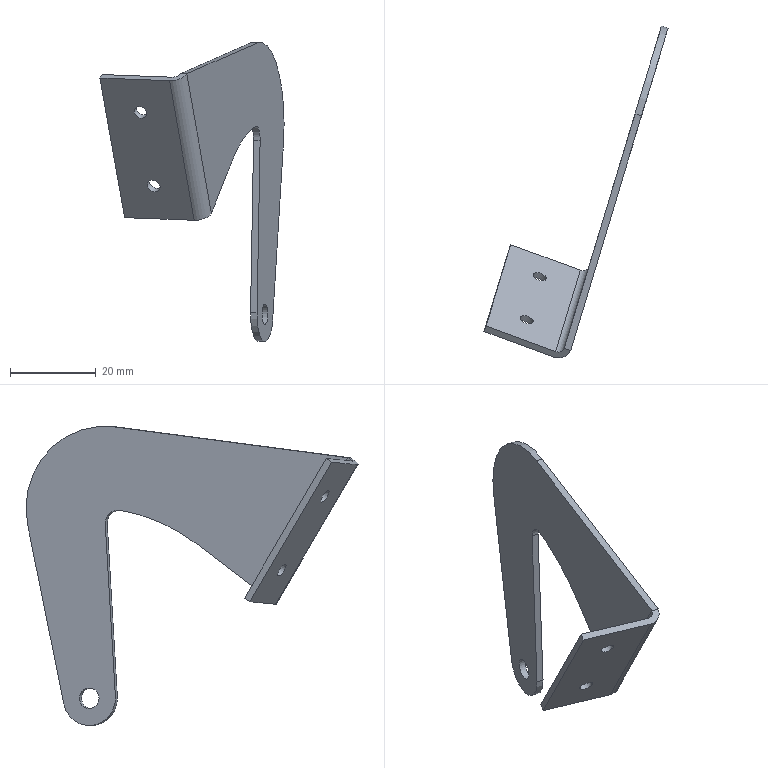Part | NX | features NG well(right door) 2 | 1 solid | 20 faces | box 42.878 x 77.32 x 69.7 mm | volume 5007 mm3 | plane 11 | cylinder 9 | commonest cylinder face diameters 3.175 x2 3.15 x1 4.763 x1 6.299 x1 6.35 x1 12.7 x1
STEP:
#1=CARTESIAN_POINT('',(90.986,-353.013,-98.868));
#2=VERTEX_POINT('',#1);
#3=CARTESIAN_POINT('',(92.506,-353.473,-98.868));
#4=VERTEX_POINT('',#3);
#5=CARTESIAN_POINT('',(90.988,-353.014,-98.868));
#6=DIRECTION('',(0.9572,-0.2893,0.));
#7=VECTOR('',#6,1000.);
#8=LINE('',#5,#7);
#9=EDGE_CURVE('',#2,#4,#8,.T.);
#10=ORIENTED_EDGE('',*,*,#9,.T.);
#11=CARTESIAN_POINT('',(88.535,-354.995,-100.462));
#12=VERTEX_POINT('',#11);
#13=CARTESIAN_POINT('',(89.514,-352.491,-98.822));
#14=DIRECTION('',(0.1509,0.4995,-0.8531));
#15=DIRECTION('',(0.,0.863,0.5053));
#16=AXIS2_PLACEMENT_3D('',#13,#14,#15);
#17=CIRCLE('',#16,3.15);
#18=EDGE_CURVE('',#4,#12,#17,.T.);
#19=ORIENTED_EDGE('',*,*,#18,.T.);
#20=CARTESIAN_POINT('',(72.328,-349.057,-99.852));
#21=VERTEX_POINT('',#20);
#22=CARTESIAN_POINT('',(90.204,-355.607,-100.524));
#23=DIRECTION('',(0.9384,-0.3438,-0.03527));
#24=VECTOR('',#23,1000.);
#25=LINE('',#22,#24);
#26=EDGE_CURVE('',#21,#12,#25,.T.);
#27=ORIENTED_EDGE('',*,*,#26,.F.);
#28=CARTESIAN_POINT('',(72.818,-347.805,-99.033));
#29=VERTEX_POINT('',#28);
#30=CARTESIAN_POINT('',(72.818,-347.805,-99.033));
#31=DIRECTION('',(-0.3109,-0.7952,-0.5206));
#32=VECTOR('',#31,1000.);
#33=LINE('',#30,#32);
#34=EDGE_CURVE('',#29,#21,#33,.T.);
#35=ORIENTED_EDGE('',*,*,#34,.F.);
#36=CARTESIAN_POINT('',(89.013,-353.738,-99.641));
#37=VERTEX_POINT('',#36);
#38=CARTESIAN_POINT('',(90.694,-354.354,-99.705));
#39=DIRECTION('',(0.9384,-0.3438,-0.03527));
#40=VECTOR('',#39,1000.);
#41=LINE('',#38,#40);
#42=EDGE_CURVE('',#29,#37,#41,.T.);
#43=ORIENTED_EDGE('',*,*,#42,.T.);
#44=CARTESIAN_POINT('',(89.502,-352.486,-98.821));
#45=DIRECTION('',(-0.1509,-0.4995,0.8531));
#46=DIRECTION('',(0.,-0.863,-0.5053));
#47=AXIS2_PLACEMENT_3D('',#44,#45,#46);
#48=CIRCLE('',#47,1.575);
#49=EDGE_CURVE('',#2,#37,#48,.F.);
#50=ORIENTED_EDGE('',*,*,#49,.F.);
#51=EDGE_LOOP('',(#10,#19,#27,#35,#43,#50));
#52=FACE_BOUND('',#51,.T.);
#53=CARTESIAN_POINT('',(90.204,-355.607,-100.524));
#54=DIRECTION('',(0.1509,0.4995,-0.8531));
#55=DIRECTION('',(0.,-0.863,-0.5053));
#56=AXIS2_PLACEMENT_3D('',#53,#54,#55);
#57=PLANE('',#56);
#58=ADVANCED_FACE('',(#52),#57,.T.);
#59=CARTESIAN_POINT('',(97.414,-337.237,-86.474));
#60=VERTEX_POINT('',#59);
#61=CARTESIAN_POINT('',(92.528,-353.405,-98.816));
#62=VERTEX_POINT('',#61);
#63=CARTESIAN_POINT('',(97.414,-337.237,-86.474));
#64=DIRECTION('',(-0.2336,-0.7729,-0.59));
#65=VECTOR('',#64,1000.);
#66=LINE('',#63,#65);
#67=EDGE_CURVE('',#60,#62,#66,.T.);
#68=ORIENTED_EDGE('',*,*,#67,.T.);
#69=CARTESIAN_POINT('',(89.513,-352.494,-98.816));
#70=DIRECTION('',(0.1707,0.5647,-0.8074));
#71=DIRECTION('',(-0.2336,-0.7729,-0.59));
#72=AXIS2_PLACEMENT_3D('',#69,#70,#71);
#73=ELLIPSE('',#72,3.16,3.15);
#74=EDGE_CURVE('',#62,#4,#73,.T.);
#75=ORIENTED_EDGE('',*,*,#74,.T.);
#76=ORIENTED_EDGE('',*,*,#9,.F.);
#77=CARTESIAN_POINT('',(91.009,-352.945,-98.815));
#78=VERTEX_POINT('',#77);
#79=CARTESIAN_POINT('',(89.501,-352.49,-98.815));
#80=DIRECTION('',(-0.1707,-0.5647,0.8074));
#81=DIRECTION('',(-0.2336,-0.7729,-0.59));
#82=AXIS2_PLACEMENT_3D('',#79,#80,#81);
#83=ELLIPSE('',#82,1.58,1.575);
#84=EDGE_CURVE('',#78,#2,#83,.F.);
#85=ORIENTED_EDGE('',*,*,#84,.F.);
#86=CARTESIAN_POINT('',(95.895,-336.777,-86.474));
#87=VERTEX_POINT('',#86);
#88=CARTESIAN_POINT('',(95.895,-336.777,-86.474));
#89=DIRECTION('',(-0.2336,-0.7729,-0.59));
#90=VECTOR('',#89,1000.);
#91=LINE('',#88,#90);
#92=EDGE_CURVE('',#87,#78,#91,.T.);
#93=ORIENTED_EDGE('',*,*,#92,.F.);
#94=CARTESIAN_POINT('',(95.895,-336.777,-86.474));
#95=DIRECTION('',(0.9572,-0.2893,0.));
#96=VECTOR('',#95,1000.);
#97=LINE('',#94,#96);
#98=EDGE_CURVE('',#87,#60,#97,.T.);
#99=ORIENTED_EDGE('',*,*,#98,.T.);
#100=EDGE_LOOP('',(#68,#75,#76,#85,#93,#99));
#101=FACE_BOUND('',#100,.T.);
#102=CARTESIAN_POINT('',(95.895,-336.777,-86.474));
#103=DIRECTION('',(0.1707,0.5647,-0.8074));
#104=DIRECTION('',(0.,-0.8195,-0.5731));
#105=AXIS2_PLACEMENT_3D('',#102,#103,#104);
#106=PLANE('',#105);
#107=ADVANCED_FACE('',(#101),#106,.T.);
#108=CARTESIAN_POINT('',(102.804,-319.401,-78.568));
#109=VERTEX_POINT('',#108);
#110=CARTESIAN_POINT('',(105.,-312.134,-122.365));
#111=DIRECTION('',(0.9572,-0.2893,0.));
#112=DIRECTION('',(0.2893,0.9572,0.));
#113=AXIS2_PLACEMENT_3D('',#110,#111,#112);
#114=CIRCLE('',#113,44.45);
#115=EDGE_CURVE('',#109,#60,#114,.T.);
#116=ORIENTED_EDGE('',*,*,#115,.T.);
#117=ORIENTED_EDGE('',*,*,#98,.F.);
#118=CARTESIAN_POINT('',(101.284,-318.942,-78.568));
#119=VERTEX_POINT('',#118);
#120=CARTESIAN_POINT('',(103.48,-311.675,-122.365));
#121=DIRECTION('',(0.9572,-0.2893,0.));
#122=DIRECTION('',(0.2893,0.9572,0.));
#123=AXIS2_PLACEMENT_3D('',#120,#121,#122);
#124=CIRCLE('',#123,44.45);
#125=EDGE_CURVE('',#119,#87,#124,.T.);
#126=ORIENTED_EDGE('',*,*,#125,.F.);
#127=CARTESIAN_POINT('',(101.284,-318.942,-78.568));
#128=DIRECTION('',(0.9572,-0.2893,0.));
#129=VECTOR('',#128,1000.);
#130=LINE('',#127,#129);
#131=EDGE_CURVE('',#109,#119,#130,.F.);
#132=ORIENTED_EDGE('',*,*,#131,.F.);
#133=EDGE_LOOP('',(#116,#117,#126,#132));
#134=FACE_BOUND('',#133,.T.);
#135=CARTESIAN_POINT('',(103.48,-311.675,-122.365));
#136=DIRECTION('',(0.9572,-0.2893,0.));
#137=DIRECTION('',(0.2893,0.9572,0.));
#138=AXIS2_PLACEMENT_3D('',#135,#136,#137);
#139=CYLINDRICAL_SURFACE('',#138,44.45);
#140=ADVANCED_FACE('',(#134),#139,.F.);
#141=CARTESIAN_POINT('',(101.647,-317.742,-121.976));
#142=VERTEX_POINT('',#141);
#143=CARTESIAN_POINT('',(102.358,-315.389,-81.891));
#144=VERTEX_POINT('',#143);
#145=CARTESIAN_POINT('',(101.647,-317.742,-121.976));
#146=DIRECTION('',(0.0177,0.05858,0.9981));
#147=VECTOR('',#146,1000.);
#148=LINE('',#145,#147);
#149=EDGE_CURVE('',#142,#144,#148,.T.);
#150=ORIENTED_EDGE('',*,*,#149,.F.);
#151=CARTESIAN_POINT('',(103.167,-318.201,-121.976));
#152=VERTEX_POINT('',#151);
#153=CARTESIAN_POINT('',(101.647,-317.742,-121.976));
#154=DIRECTION('',(0.9572,-0.2893,0.));
#155=VECTOR('',#154,1000.);
#156=LINE('',#153,#155);
#157=EDGE_CURVE('',#142,#152,#156,.T.);
#158=ORIENTED_EDGE('',*,*,#157,.T.);
#159=CARTESIAN_POINT('',(103.878,-315.849,-81.891));
#160=VERTEX_POINT('',#159);
#161=CARTESIAN_POINT('',(103.167,-318.201,-121.976));
#162=DIRECTION('',(0.0177,0.05858,0.9981));
#163=VECTOR('',#162,1000.);
#164=LINE('',#161,#163);
#165=EDGE_CURVE('',#152,#160,#164,.T.);
#166=ORIENTED_EDGE('',*,*,#165,.T.);
#167=CARTESIAN_POINT('',(103.878,-315.849,-81.891));
#168=DIRECTION('',(-0.9572,0.2893,0.));
#169=VECTOR('',#168,1000.);
#170=LINE('',#167,#169);
#171=EDGE_CURVE('',#144,#160,#170,.F.);
#172=ORIENTED_EDGE('',*,*,#171,.F.);
#173=EDGE_LOOP('',(#150,#158,#166,#172));
#174=FACE_BOUND('',#173,.T.);
#175=CARTESIAN_POINT('',(101.647,-317.742,-121.976));
#176=DIRECTION('',(-0.2887,-0.9555,0.0612));
#177=DIRECTION('',(0.9572,-0.2893,0.));
#178=AXIS2_PLACEMENT_3D('',#175,#176,#177);
#179=PLANE('',#178);
#180=ADVANCED_FACE('',(#174),#179,.T.);
#181=CARTESIAN_POINT('',(106.797,-306.186,-123.674));
#182=VERTEX_POINT('',#181);
#183=CARTESIAN_POINT('',(105.,-312.134,-122.365));
#184=DIRECTION('',(-0.9572,0.2893,0.));
#185=DIRECTION('',(0.2893,0.9572,0.));
#186=AXIS2_PLACEMENT_3D('',#183,#184,#185);
#187=CIRCLE('',#186,6.35);
#188=EDGE_CURVE('',#182,#152,#187,.T.);
#189=ORIENTED_EDGE('',*,*,#188,.T.);
#190=ORIENTED_EDGE('',*,*,#157,.F.);
#191=CARTESIAN_POINT('',(105.278,-305.727,-123.674));
#192=VERTEX_POINT('',#191);
#193=CARTESIAN_POINT('',(103.48,-311.675,-122.365));
#194=DIRECTION('',(-0.9572,0.2893,0.));
#195=DIRECTION('',(0.2893,0.9572,0.));
#196=AXIS2_PLACEMENT_3D('',#193,#194,#195);
#197=CIRCLE('',#196,6.35);
#198=EDGE_CURVE('',#192,#142,#197,.T.);
#199=ORIENTED_EDGE('',*,*,#198,.F.);
#200=CARTESIAN_POINT('',(105.278,-305.727,-123.674));
#201=DIRECTION('',(0.9572,-0.2893,0.));
#202=VECTOR('',#201,1000.);
#203=LINE('',#200,#202);
#204=EDGE_CURVE('',#192,#182,#203,.T.);
#205=ORIENTED_EDGE('',*,*,#204,.T.);
#206=EDGE_LOOP('',(#189,#190,#199,#205));
#207=FACE_BOUND('',#206,.T.);
#208=CARTESIAN_POINT('',(103.48,-311.675,-122.365));
#209=DIRECTION('',(0.9572,-0.2893,0.));
#210=DIRECTION('',(0.2893,0.9572,0.));
#211=AXIS2_PLACEMENT_3D('',#208,#209,#210);
#212=CYLINDRICAL_SURFACE('',#211,6.35);
#213=ADVANCED_FACE('',(#207),#212,.T.);
#214=CARTESIAN_POINT('',(109.338,-297.78,-81.992));
#215=VERTEX_POINT('',#214);
#216=CARTESIAN_POINT('',(106.797,-306.186,-123.674));
#217=DIRECTION('',(-0.05963,-0.1973,-0.9785));
#218=VECTOR('',#217,1000.);
#219=LINE('',#216,#218);
#220=EDGE_CURVE('',#215,#182,#219,.T.);
#221=ORIENTED_EDGE('',*,*,#220,.T.);
#222=ORIENTED_EDGE('',*,*,#204,.F.);
#223=CARTESIAN_POINT('',(107.818,-297.321,-81.992));
#224=VERTEX_POINT('',#223);
#225=CARTESIAN_POINT('',(105.278,-305.727,-123.674));
#226=DIRECTION('',(-0.05963,-0.1973,-0.9785));
#227=VECTOR('',#226,1000.);
#228=LINE('',#225,#227);
#229=EDGE_CURVE('',#224,#192,#228,.T.);
#230=ORIENTED_EDGE('',*,*,#229,.F.);
#231=CARTESIAN_POINT('',(107.818,-297.321,-81.992));
#232=DIRECTION('',(0.9572,-0.2893,0.));
#233=VECTOR('',#232,1000.);
#234=LINE('',#231,#233);
#235=EDGE_CURVE('',#224,#215,#234,.T.);
#236=ORIENTED_EDGE('',*,*,#235,.T.);
#237=EDGE_LOOP('',(#221,#222,#230,#236));
#238=FACE_BOUND('',#237,.T.);
#239=CARTESIAN_POINT('',(105.278,-305.727,-123.674));
#240=DIRECTION('',(0.2831,0.9367,-0.2062));
#241=DIRECTION('',(-0.9572,0.2893,0.));
#242=AXIS2_PLACEMENT_3D('',#239,#240,#241);
#243=PLANE('',#242);
#244=ADVANCED_FACE('',(#238),#243,.T.);
#245=CARTESIAN_POINT('',(103.255,-317.908,-59.165));
#246=VERTEX_POINT('',#245);
#247=CARTESIAN_POINT('',(103.945,-315.624,-78.065));
#248=DIRECTION('',(-0.9572,0.2893,0.));
#249=DIRECTION('',(0.2893,0.9572,0.));
#250=AXIS2_PLACEMENT_3D('',#247,#248,#249);
#251=CIRCLE('',#250,19.05);
#252=EDGE_CURVE('',#246,#215,#251,.T.);
#253=ORIENTED_EDGE('',*,*,#252,.T.);
#254=ORIENTED_EDGE('',*,*,#235,.F.);
#255=CARTESIAN_POINT('',(101.736,-317.449,-59.165));
#256=VERTEX_POINT('',#255);
#257=CARTESIAN_POINT('',(102.426,-315.165,-78.065));
#258=DIRECTION('',(-0.9572,0.2893,0.));
#259=DIRECTION('',(0.2893,0.9572,0.));
#260=AXIS2_PLACEMENT_3D('',#257,#258,#259);
#261=CIRCLE('',#260,19.05);
#262=EDGE_CURVE('',#256,#224,#261,.T.);
#263=ORIENTED_EDGE('',*,*,#262,.F.);
#264=CARTESIAN_POINT('',(101.736,-317.449,-59.165));
#265=DIRECTION('',(0.9572,-0.2893,0.));
#266=VECTOR('',#265,1000.);
#267=LINE('',#264,#266);
#268=EDGE_CURVE('',#256,#246,#267,.T.);
#269=ORIENTED_EDGE('',*,*,#268,.T.);
#270=EDGE_LOOP('',(#253,#254,#263,#269));
#271=FACE_BOUND('',#270,.T.);
#272=CARTESIAN_POINT('',(102.426,-315.165,-78.065));
#273=DIRECTION('',(0.9572,-0.2893,0.));
#274=DIRECTION('',(0.2893,0.9572,0.));
#275=AXIS2_PLACEMENT_3D('',#272,#273,#274);
#276=CYLINDRICAL_SURFACE('',#275,19.05);
#277=ADVANCED_FACE('',(#271),#276,.T.);
#278=CARTESIAN_POINT('',(85.235,-372.043,-66.365));
#279=VERTEX_POINT('',#278);
#280=CARTESIAN_POINT('',(86.756,-372.503,-66.365));
#281=VERTEX_POINT('',#280);
#282=CARTESIAN_POINT('',(85.237,-372.044,-66.365));
#283=DIRECTION('',(0.9572,-0.2893,0.));
#284=VECTOR('',#283,1000.);
#285=LINE('',#282,#284);
#286=EDGE_CURVE('',#279,#281,#285,.T.);
#287=ORIENTED_EDGE('',*,*,#286,.T.);
#288=CARTESIAN_POINT('',(86.784,-372.412,-66.353));
#289=VERTEX_POINT('',#288);
#290=CARTESIAN_POINT('',(83.769,-371.501,-66.353));
#291=DIRECTION('',(-0.03623,-0.1199,0.9921));
#292=DIRECTION('',(0.287,0.9497,0.1253));
#293=AXIS2_PLACEMENT_3D('',#290,#291,#292);
#294=ELLIPSE('',#293,3.455,3.15);
#295=EDGE_CURVE('',#281,#289,#294,.T.);
#296=ORIENTED_EDGE('',*,*,#295,.T.);
#297=CARTESIAN_POINT('',(86.757,-372.503,-66.365));
#298=DIRECTION('',(0.287,0.9497,0.1253));
#299=VECTOR('',#298,1000.);
#300=LINE('',#297,#299);
#301=EDGE_CURVE('',#289,#246,#300,.T.);
#302=ORIENTED_EDGE('',*,*,#301,.T.);
#303=ORIENTED_EDGE('',*,*,#268,.F.);
#304=CARTESIAN_POINT('',(85.265,-371.952,-66.353));
#305=VERTEX_POINT('',#304);
#306=CARTESIAN_POINT('',(85.237,-372.044,-66.365));
#307=DIRECTION('',(0.287,0.9497,0.1253));
#308=VECTOR('',#307,1000.);
#309=LINE('',#306,#308);
#310=EDGE_CURVE('',#305,#256,#309,.T.);
#311=ORIENTED_EDGE('',*,*,#310,.F.);
#312=CARTESIAN_POINT('',(83.758,-371.496,-66.353));
#313=DIRECTION('',(0.03623,0.1199,-0.9921));
#314=DIRECTION('',(0.287,0.9497,0.1253));
#315=AXIS2_PLACEMENT_3D('',#312,#313,#314);
#316=ELLIPSE('',#315,1.727,1.575);
#317=EDGE_CURVE('',#279,#305,#316,.F.);
#318=ORIENTED_EDGE('',*,*,#317,.F.);
#319=EDGE_LOOP('',(#287,#296,#302,#303,#311,#318));
#320=FACE_BOUND('',#319,.T.);
#321=CARTESIAN_POINT('',(85.237,-372.044,-66.365));
#322=DIRECTION('',(-0.03623,-0.1199,0.9921));
#323=DIRECTION('',(0.,0.9928,0.12));
#324=AXIS2_PLACEMENT_3D('',#321,#322,#323);
#325=PLANE('',#324);
#326=ADVANCED_FACE('',(#320),#325,.T.);
#327=CARTESIAN_POINT('',(82.784,-374.025,-67.959));
#328=VERTEX_POINT('',#327);
#329=CARTESIAN_POINT('',(66.578,-368.087,-67.35));
#330=VERTEX_POINT('',#329);
#331=CARTESIAN_POINT('',(84.454,-374.637,-68.022));
#332=DIRECTION('',(-0.9384,0.3438,0.03527));
#333=VECTOR('',#332,1000.);
#334=LINE('',#331,#333);
#335=EDGE_CURVE('',#328,#330,#334,.T.);
#336=ORIENTED_EDGE('',*,*,#335,.F.);
#337=CARTESIAN_POINT('',(83.764,-371.521,-66.32));
#338=DIRECTION('',(-0.1509,-0.4995,0.8531));
#339=DIRECTION('',(0.,-0.863,-0.5053));
#340=AXIS2_PLACEMENT_3D('',#337,#338,#339);
#341=CIRCLE('',#340,3.15);
#342=EDGE_CURVE('',#328,#281,#341,.T.);
#343=ORIENTED_EDGE('',*,*,#342,.T.);
#344=ORIENTED_EDGE('',*,*,#286,.F.);
#345=CARTESIAN_POINT('',(83.262,-372.769,-67.139));
#346=VERTEX_POINT('',#345);
#347=CARTESIAN_POINT('',(83.752,-371.516,-66.319));
#348=DIRECTION('',(0.1509,0.4995,-0.8531));
#349=DIRECTION('',(0.,0.863,0.5053));
#350=AXIS2_PLACEMENT_3D('',#347,#348,#349);
#351=CIRCLE('',#350,1.575);
#352=EDGE_CURVE('',#346,#279,#351,.F.);
#353=ORIENTED_EDGE('',*,*,#352,.F.);
#354=CARTESIAN_POINT('',(67.067,-366.835,-66.53));
#355=VERTEX_POINT('',#354);
#356=CARTESIAN_POINT('',(84.943,-373.385,-67.202));
#357=DIRECTION('',(-0.9384,0.3438,0.03527));
#358=VECTOR('',#357,1000.);
#359=LINE('',#356,#358);
#360=EDGE_CURVE('',#346,#355,#359,.T.);
#361=ORIENTED_EDGE('',*,*,#360,.T.);
#362=CARTESIAN_POINT('',(67.067,-366.835,-66.53));
#363=DIRECTION('',(-0.3109,-0.7952,-0.5206));
#364=VECTOR('',#363,1000.);
#365=LINE('',#362,#364);
#366=EDGE_CURVE('',#355,#330,#365,.T.);
#367=ORIENTED_EDGE('',*,*,#366,.T.);
#368=EDGE_LOOP('',(#336,#343,#344,#353,#361,#367));
#369=FACE_BOUND('',#368,.T.);
#370=CARTESIAN_POINT('',(85.237,-372.044,-66.365));
#371=DIRECTION('',(-0.1509,-0.4995,0.8531));
#372=DIRECTION('',(0.,0.863,0.5053));
#373=AXIS2_PLACEMENT_3D('',#370,#371,#372);
#374=PLANE('',#373);
#375=ADVANCED_FACE('',(#369),#374,.T.);
#376=CARTESIAN_POINT('',(104.169,-309.396,-122.365));
#377=VERTEX_POINT('',#376);
#378=CARTESIAN_POINT('',(103.48,-311.675,-122.365));
#379=DIRECTION('',(-0.9572,0.2893,0.));
#380=DIRECTION('',(0.2893,0.9572,0.));
#381=AXIS2_PLACEMENT_3D('',#378,#379,#380);
#382=CIRCLE('',#381,2.381);
#383=EDGE_CURVE('',#377,#377,#382,.T.);
#384=ORIENTED_EDGE('',*,*,#383,.F.);
#385=EDGE_LOOP('',(#384));
#386=FACE_BOUND('',#385,.T.);
#387=ORIENTED_EDGE('',*,*,#310,.T.);
#388=ORIENTED_EDGE('',*,*,#262,.T.);
#389=ORIENTED_EDGE('',*,*,#229,.T.);
#390=ORIENTED_EDGE('',*,*,#198,.T.);
#391=ORIENTED_EDGE('',*,*,#149,.T.);
#392=CARTESIAN_POINT('',(101.441,-318.423,-81.696));
#393=DIRECTION('',(-0.9572,0.2893,0.));
#394=DIRECTION('',(0.2893,0.9572,0.));
#395=AXIS2_PLACEMENT_3D('',#392,#393,#394);
#396=CIRCLE('',#395,3.175);
#397=EDGE_CURVE('',#119,#144,#396,.T.);
#398=ORIENTED_EDGE('',*,*,#397,.F.);
#399=ORIENTED_EDGE('',*,*,#125,.T.);
#400=ORIENTED_EDGE('',*,*,#92,.T.);
#401=CARTESIAN_POINT('',(97.437,-331.675,-135.144));
#402=DIRECTION('',(0.1509,0.4995,-0.8531));
#403=VECTOR('',#402,1000.);
#404=LINE('',#401,#403);
#405=EDGE_CURVE('',#305,#78,#404,.T.);
#406=ORIENTED_EDGE('',*,*,#405,.F.);
#407=EDGE_LOOP('',(#387,#388,#389,#390,#391,#398,#399,#400,#406));
#408=FACE_BOUND('',#407,.T.);
#409=CARTESIAN_POINT('',(103.48,-311.675,-122.365));
#410=DIRECTION('',(0.9572,-0.2893,0.));
#411=DIRECTION('',(0.2893,0.9572,0.));
#412=AXIS2_PLACEMENT_3D('',#409,#410,#411);
#413=PLANE('',#412);
#414=ADVANCED_FACE('',(#386,#408),#413,.F.);
#415=CARTESIAN_POINT('',(105.689,-309.855,-122.365));
#416=VERTEX_POINT('',#415);
#417=CARTESIAN_POINT('',(105.,-312.134,-122.365));
#418=DIRECTION('',(-0.9572,0.2893,0.));
#419=DIRECTION('',(0.2893,0.9572,0.));
#420=AXIS2_PLACEMENT_3D('',#417,#418,#419);
#421=CIRCLE('',#420,2.381);
#422=EDGE_CURVE('',#416,#416,#421,.T.);
#423=ORIENTED_EDGE('',*,*,#422,.T.);
#424=EDGE_LOOP('',(#423));
#425=FACE_BOUND('',#424,.T.);
#426=ORIENTED_EDGE('',*,*,#301,.F.);
#427=CARTESIAN_POINT('',(92.529,-353.402,-98.822));
#428=DIRECTION('',(-0.1509,-0.4995,0.8531));
#429=VECTOR('',#428,1000.);
#430=LINE('',#427,#429);
#431=EDGE_CURVE('',#289,#62,#430,.F.);
#432=ORIENTED_EDGE('',*,*,#431,.T.);
#433=ORIENTED_EDGE('',*,*,#67,.F.);
#434=ORIENTED_EDGE('',*,*,#115,.F.);
#435=CARTESIAN_POINT('',(102.961,-318.882,-81.696));
#436=DIRECTION('',(-0.9572,0.2893,0.));
#437=DIRECTION('',(0.2893,0.9572,0.));
#438=AXIS2_PLACEMENT_3D('',#435,#436,#437);
#439=CIRCLE('',#438,3.175);
#440=EDGE_CURVE('',#160,#109,#439,.F.);
#441=ORIENTED_EDGE('',*,*,#440,.F.);
#442=ORIENTED_EDGE('',*,*,#165,.F.);
#443=ORIENTED_EDGE('',*,*,#188,.F.);
#444=ORIENTED_EDGE('',*,*,#220,.F.);
#445=ORIENTED_EDGE('',*,*,#252,.F.);
#446=EDGE_LOOP('',(#426,#432,#433,#434,#441,#442,#443,#444,#445));
#447=FACE_BOUND('',#446,.T.);
#448=CARTESIAN_POINT('',(105.,-312.134,-122.365));
#449=DIRECTION('',(0.9572,-0.2893,0.));
#450=DIRECTION('',(0.2893,0.9572,0.));
#451=AXIS2_PLACEMENT_3D('',#448,#449,#450);
#452=PLANE('',#451);
#453=ADVANCED_FACE('',(#425,#447),#452,.T.);
#454=ORIENTED_EDGE('',*,*,#383,.T.);
#455=EDGE_LOOP('',(#454));
#456=FACE_BOUND('',#455,.T.);
#457=ORIENTED_EDGE('',*,*,#422,.F.);
#458=EDGE_LOOP('',(#457));
#459=FACE_BOUND('',#458,.T.);
#460=CARTESIAN_POINT('',(103.48,-311.675,-122.365));
#461=DIRECTION('',(0.9572,-0.2893,0.));
#462=DIRECTION('',(0.2893,0.9572,0.));
#463=AXIS2_PLACEMENT_3D('',#460,#461,#462);
#464=CYLINDRICAL_SURFACE('',#463,2.381);
#465=ADVANCED_FACE('',(#456,#459),#464,.F.);
#466=ORIENTED_EDGE('',*,*,#397,.T.);
#467=ORIENTED_EDGE('',*,*,#171,.T.);
#468=ORIENTED_EDGE('',*,*,#440,.T.);
#469=ORIENTED_EDGE('',*,*,#131,.T.);
#470=EDGE_LOOP('',(#466,#467,#468,#469));
#471=FACE_BOUND('',#470,.T.);
#472=CARTESIAN_POINT('',(101.441,-318.423,-81.696));
#473=DIRECTION('',(0.9572,-0.2893,0.));
#474=DIRECTION('',(0.2893,0.9572,0.));
#475=AXIS2_PLACEMENT_3D('',#472,#473,#474);
#476=CYLINDRICAL_SURFACE('',#475,3.175);
#477=ADVANCED_FACE('',(#471),#476,.F.);
#478=CARTESIAN_POINT('',(76.523,-364.437,-75.841));
#479=VERTEX_POINT('',#478);
#480=CARTESIAN_POINT('',(76.523,-365.306,-74.512));
#481=DIRECTION('',(-0.3109,-0.7952,-0.5206));
#482=DIRECTION('',(0.,0.5477,-0.8366));
#483=AXIS2_PLACEMENT_3D('',#480,#481,#482);
#484=CIRCLE('',#483,1.587);
#485=EDGE_CURVE('',#479,#479,#484,.T.);
#486=ORIENTED_EDGE('',*,*,#485,.T.);
#487=EDGE_LOOP('',(#486));
#488=FACE_BOUND('',#487,.T.);
#489=CARTESIAN_POINT('',(79.557,-354.397,-92.987));
#490=VERTEX_POINT('',#489);
#491=CARTESIAN_POINT('',(79.557,-355.267,-91.659));
#492=DIRECTION('',(-0.3109,-0.7952,-0.5206));
#493=DIRECTION('',(0.,0.5477,-0.8366));
#494=AXIS2_PLACEMENT_3D('',#491,#492,#493);
#495=CIRCLE('',#494,1.587);
#496=EDGE_CURVE('',#490,#490,#495,.T.);
#497=ORIENTED_EDGE('',*,*,#496,.T.);
#498=EDGE_LOOP('',(#497));
#499=FACE_BOUND('',#498,.T.);
#500=ORIENTED_EDGE('',*,*,#42,.F.);
#501=CARTESIAN_POINT('',(67.067,-366.835,-66.53));
#502=DIRECTION('',(0.1509,0.4995,-0.8531));
#503=VECTOR('',#502,1000.);
#504=LINE('',#501,#503);
#505=EDGE_CURVE('',#355,#29,#504,.T.);
#506=ORIENTED_EDGE('',*,*,#505,.F.);
#507=ORIENTED_EDGE('',*,*,#360,.F.);
#508=CARTESIAN_POINT('',(83.262,-372.769,-67.139));
#509=DIRECTION('',(0.1509,0.4995,-0.8531));
#510=VECTOR('',#509,1000.);
#511=LINE('',#508,#510);
#512=EDGE_CURVE('',#37,#346,#511,.F.);
#513=ORIENTED_EDGE('',*,*,#512,.F.);
#514=EDGE_LOOP('',(#500,#506,#507,#513));
#515=FACE_BOUND('',#514,.T.);
#516=CARTESIAN_POINT('',(84.943,-373.385,-67.202));
#517=DIRECTION('',(0.3109,0.7952,0.5206));
#518=DIRECTION('',(0.,0.5477,-0.8366));
#519=AXIS2_PLACEMENT_3D('',#516,#517,#518);
#520=PLANE('',#519);
#521=ADVANCED_FACE('',(#488,#499,#515),#520,.T.);
#522=CARTESIAN_POINT('',(66.578,-368.087,-67.35));
#523=DIRECTION('',(0.1509,0.4995,-0.8531));
#524=VECTOR('',#523,1000.);
#525=LINE('',#522,#524);
#526=EDGE_CURVE('',#330,#21,#525,.T.);
#527=ORIENTED_EDGE('',*,*,#526,.F.);
#528=ORIENTED_EDGE('',*,*,#366,.F.);
#529=ORIENTED_EDGE('',*,*,#505,.T.);
#530=ORIENTED_EDGE('',*,*,#34,.T.);
#531=EDGE_LOOP('',(#527,#528,#529,#530));
#532=FACE_BOUND('',#531,.T.);
#533=CARTESIAN_POINT('',(67.067,-366.835,-66.53));
#534=DIRECTION('',(0.9384,-0.3438,-0.03527));
#535=DIRECTION('',(0.344,0.939,0.));
#536=AXIS2_PLACEMENT_3D('',#533,#534,#535);
#537=PLANE('',#536);
#538=ADVANCED_FACE('',(#532),#537,.F.);
#539=CARTESIAN_POINT('',(76.033,-367.428,-74.004));
#540=VERTEX_POINT('',#539);
#541=CARTESIAN_POINT('',(76.033,-366.559,-75.332));
#542=DIRECTION('',(0.3109,0.7952,0.5206));
#543=DIRECTION('',(0.,-0.5477,0.8366));
#544=AXIS2_PLACEMENT_3D('',#541,#542,#543);
#545=CIRCLE('',#544,1.587);
#546=EDGE_CURVE('',#540,#540,#545,.T.);
#547=ORIENTED_EDGE('',*,*,#546,.T.);
#548=EDGE_LOOP('',(#547));
#549=FACE_BOUND('',#548,.T.);
#550=CARTESIAN_POINT('',(79.067,-357.389,-91.151));
#551=VERTEX_POINT('',#550);
#552=CARTESIAN_POINT('',(79.067,-356.519,-92.479));
#553=DIRECTION('',(0.3109,0.7952,0.5206));
#554=DIRECTION('',(0.,-0.5477,0.8366));
#555=AXIS2_PLACEMENT_3D('',#552,#553,#554);
#556=CIRCLE('',#555,1.587);
#557=EDGE_CURVE('',#551,#551,#556,.T.);
#558=ORIENTED_EDGE('',*,*,#557,.T.);
#559=EDGE_LOOP('',(#558));
#560=FACE_BOUND('',#559,.T.);
#561=ORIENTED_EDGE('',*,*,#26,.T.);
#562=CARTESIAN_POINT('',(82.784,-374.025,-67.959));
#563=DIRECTION('',(-0.1509,-0.4995,0.8531));
#564=VECTOR('',#563,1000.);
#565=LINE('',#562,#564);
#566=EDGE_CURVE('',#12,#328,#565,.T.);
#567=ORIENTED_EDGE('',*,*,#566,.T.);
#568=ORIENTED_EDGE('',*,*,#335,.T.);
#569=ORIENTED_EDGE('',*,*,#526,.T.);
#570=EDGE_LOOP('',(#561,#567,#568,#569));
#571=FACE_BOUND('',#570,.T.);
#572=CARTESIAN_POINT('',(84.454,-374.637,-68.022));
#573=DIRECTION('',(0.3109,0.7952,0.5206));
#574=DIRECTION('',(0.,0.5477,-0.8366));
#575=AXIS2_PLACEMENT_3D('',#572,#573,#574);
#576=PLANE('',#575);
#577=ADVANCED_FACE('',(#549,#560,#571),#576,.F.);
#578=ORIENTED_EDGE('',*,*,#352,.T.);
#579=ORIENTED_EDGE('',*,*,#317,.T.);
#580=ORIENTED_EDGE('',*,*,#405,.T.);
#581=ORIENTED_EDGE('',*,*,#84,.T.);
#582=ORIENTED_EDGE('',*,*,#49,.T.);
#583=ORIENTED_EDGE('',*,*,#512,.T.);
#584=EDGE_LOOP('',(#578,#579,#580,#581,#582,#583));
#585=FACE_BOUND('',#584,.T.);
#586=CARTESIAN_POINT('',(95.929,-331.219,-135.144));
#587=DIRECTION('',(0.1509,0.4995,-0.8531));
#588=DIRECTION('',(0.,-0.863,-0.5053));
#589=AXIS2_PLACEMENT_3D('',#586,#587,#588);
#590=CYLINDRICAL_SURFACE('',#589,1.575);
#591=ADVANCED_FACE('',(#585),#590,.F.);
#592=ORIENTED_EDGE('',*,*,#496,.F.);
#593=EDGE_LOOP('',(#592));
#594=FACE_BOUND('',#593,.T.);
#595=ORIENTED_EDGE('',*,*,#557,.F.);
#596=EDGE_LOOP('',(#595));
#597=FACE_BOUND('',#596,.T.);
#598=CARTESIAN_POINT('',(79.557,-355.267,-91.659));
#599=DIRECTION('',(-0.3109,-0.7952,-0.5206));
#600=DIRECTION('',(0.,0.5477,-0.8366));
#601=AXIS2_PLACEMENT_3D('',#598,#599,#600);
#602=CYLINDRICAL_SURFACE('',#601,1.587);
#603=ADVANCED_FACE('',(#594,#597),#602,.F.);
#604=ORIENTED_EDGE('',*,*,#485,.F.);
#605=EDGE_LOOP('',(#604));
#606=FACE_BOUND('',#605,.T.);
#607=ORIENTED_EDGE('',*,*,#546,.F.);
#608=EDGE_LOOP('',(#607));
#609=FACE_BOUND('',#608,.T.);
#610=CARTESIAN_POINT('',(76.523,-365.306,-74.512));
#611=DIRECTION('',(-0.3109,-0.7952,-0.5206));
#612=DIRECTION('',(0.,0.5477,-0.8366));
#613=AXIS2_PLACEMENT_3D('',#610,#611,#612);
#614=CYLINDRICAL_SURFACE('',#613,1.587);
#615=ADVANCED_FACE('',(#606,#609),#614,.F.);
#616=ORIENTED_EDGE('',*,*,#74,.F.);
#617=ORIENTED_EDGE('',*,*,#431,.F.);
#618=ORIENTED_EDGE('',*,*,#295,.F.);
#619=ORIENTED_EDGE('',*,*,#342,.F.);
#620=ORIENTED_EDGE('',*,*,#566,.F.);
#621=ORIENTED_EDGE('',*,*,#18,.F.);
#622=EDGE_LOOP('',(#616,#617,#618,#619,#620,#621));
#623=FACE_BOUND('',#622,.T.);
#624=CARTESIAN_POINT('',(83.764,-371.521,-66.32));
#625=DIRECTION('',(0.1509,0.4995,-0.8531));
#626=DIRECTION('',(0.,0.863,0.5053));
#627=AXIS2_PLACEMENT_3D('',#624,#625,#626);
#628=CYLINDRICAL_SURFACE('',#627,3.15);
#629=ADVANCED_FACE('',(#623),#628,.T.);
#630=CLOSED_SHELL('',(#58,#107,#140,#180,#213,#244,#277,#326,#375,#414,#453,#465,#477,#521,#538,#577,#591,#603,#615,#629));
#631=MANIFOLD_SOLID_BREP('',#630);
#632=(LENGTH_UNIT()NAMED_UNIT(*)SI_UNIT(.MILLI.,.METRE.));
#633=UNCERTAINTY_MEASURE_WITH_UNIT(LENGTH_MEASURE(0.00001),#632,'','');
#634=(NAMED_UNIT(*)PLANE_ANGLE_UNIT()SI_UNIT($,.RADIAN.));
#635=(NAMED_UNIT(*)SI_UNIT($,.STERADIAN.)SOLID_ANGLE_UNIT());
#636=(GEOMETRIC_REPRESENTATION_CONTEXT(3)GLOBAL_UNCERTAINTY_ASSIGNED_CONTEXT((#633))GLOBAL_UNIT_ASSIGNED_CONTEXT((#632,#634,#635))REPRESENTATION_CONTEXT('',''));
#637=ADVANCED_BREP_SHAPE_REPRESENTATION('',(#631),#636);